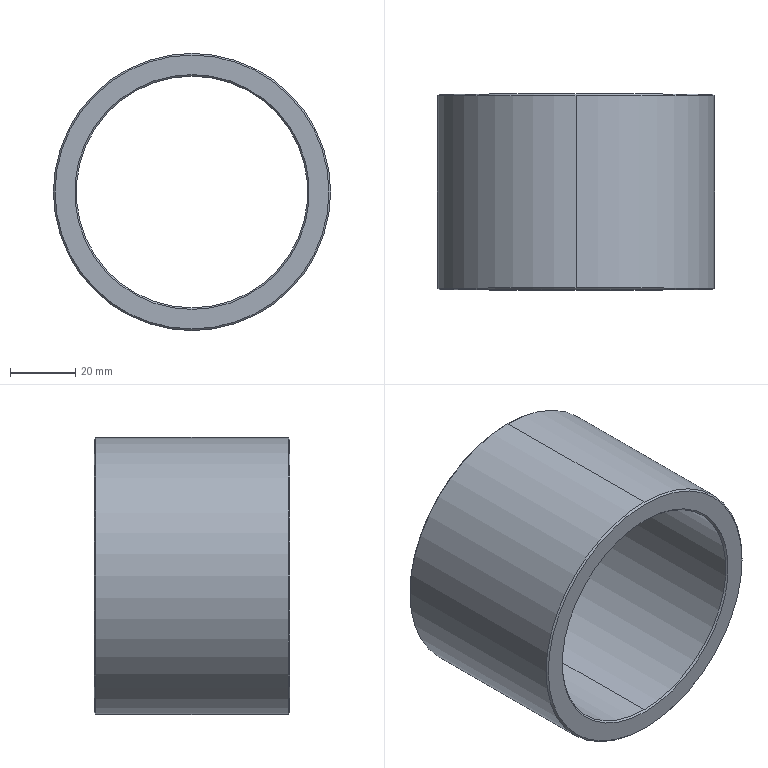Part | SolidWorks | features Chamfer 1, Extrusion 1 | 1 solid | 14 faces | box 85 x 60 x 85 mm | volume 102796 mm3 | cone 8 | cylinder 4 | plane 2 | commonest cylinder face diameters 71 x2 85 x2
STEP:
#1=CARTESIAN_POINT('',(0.,0.5,35.5));
#2=VERTEX_POINT('',#1);
#3=CARTESIAN_POINT('',(0.,0.5,-35.5));
#4=VERTEX_POINT('',#3);
#5=CARTESIAN_POINT('',(0.,0.5,0.));
#6=DIRECTION('',(0.,-1.,0.));
#7=DIRECTION('',(0.,0.,1.));
#8=AXIS2_PLACEMENT_3D('',#5,#6,#7);
#9=CIRCLE('',#8,35.5);
#10=EDGE_CURVE('',#2,#4,#9,.T.);
#11=ORIENTED_EDGE('',*,*,#10,.F.);
#12=CARTESIAN_POINT('',(0.,0.,36.));
#13=VERTEX_POINT('',#12);
#14=CARTESIAN_POINT('',(0.,0.,36.));
#15=DIRECTION('',(0.,-0.7071,0.7071));
#16=VECTOR('',#15,1000.);
#17=LINE('',#14,#16);
#18=EDGE_CURVE('',#2,#13,#17,.T.);
#19=ORIENTED_EDGE('',*,*,#18,.T.);
#20=CARTESIAN_POINT('',(0.,0.,-36.));
#21=VERTEX_POINT('',#20);
#22=CARTESIAN_POINT('',(0.,0.,0.));
#23=DIRECTION('',(0.,1.,0.));
#24=DIRECTION('',(0.,0.,1.));
#25=AXIS2_PLACEMENT_3D('',#22,#23,#24);
#26=CIRCLE('',#25,36.);
#27=EDGE_CURVE('',#21,#13,#26,.T.);
#28=ORIENTED_EDGE('',*,*,#27,.F.);
#29=CARTESIAN_POINT('',(0.,0.,-36.));
#30=DIRECTION('',(0.,-0.7071,-0.7071));
#31=VECTOR('',#30,1000.);
#32=LINE('',#29,#31);
#33=EDGE_CURVE('',#4,#21,#32,.T.);
#34=ORIENTED_EDGE('',*,*,#33,.F.);
#35=EDGE_LOOP('',(#11,#19,#28,#34));
#36=FACE_OUTER_BOUND('',#35,.T.);
#37=CARTESIAN_POINT('',(0.,0.,0.));
#38=DIRECTION('',(0.,-1.,0.));
#39=DIRECTION('',(0.,0.,-1.));
#40=AXIS2_PLACEMENT_3D('',#37,#38,#39);
#41=CONICAL_SURFACE('',#40,36.,0.7854);
#42=ADVANCED_FACE('',(#36),#41,.F.);
#43=CARTESIAN_POINT('',(0.,59.5,-35.5));
#44=VERTEX_POINT('',#43);
#45=CARTESIAN_POINT('',(0.,59.5,35.5));
#46=VERTEX_POINT('',#45);
#47=CARTESIAN_POINT('',(0.,59.5,0.));
#48=DIRECTION('',(0.,1.,0.));
#49=DIRECTION('',(0.,0.,1.));
#50=AXIS2_PLACEMENT_3D('',#47,#48,#49);
#51=CIRCLE('',#50,35.5);
#52=EDGE_CURVE('',#44,#46,#51,.T.);
#53=ORIENTED_EDGE('',*,*,#52,.F.);
#54=CARTESIAN_POINT('',(0.,60.,-36.));
#55=VERTEX_POINT('',#54);
#56=CARTESIAN_POINT('',(0.,59.5,-35.5));
#57=DIRECTION('',(0.,0.7071,-0.7071));
#58=VECTOR('',#57,1000.);
#59=LINE('',#56,#58);
#60=EDGE_CURVE('',#44,#55,#59,.T.);
#61=ORIENTED_EDGE('',*,*,#60,.T.);
#62=CARTESIAN_POINT('',(0.,60.,36.));
#63=VERTEX_POINT('',#62);
#64=CARTESIAN_POINT('',(0.,60.,0.));
#65=DIRECTION('',(0.,-1.,0.));
#66=DIRECTION('',(0.,0.,1.));
#67=AXIS2_PLACEMENT_3D('',#64,#65,#66);
#68=CIRCLE('',#67,36.);
#69=EDGE_CURVE('',#63,#55,#68,.T.);
#70=ORIENTED_EDGE('',*,*,#69,.F.);
#71=CARTESIAN_POINT('',(0.,59.5,35.5));
#72=DIRECTION('',(0.,0.7071,0.7071));
#73=VECTOR('',#72,1000.);
#74=LINE('',#71,#73);
#75=EDGE_CURVE('',#46,#63,#74,.T.);
#76=ORIENTED_EDGE('',*,*,#75,.F.);
#77=EDGE_LOOP('',(#53,#61,#70,#76));
#78=FACE_OUTER_BOUND('',#77,.T.);
#79=CARTESIAN_POINT('',(0.,59.5,0.));
#80=DIRECTION('',(0.,1.,0.));
#81=DIRECTION('',(0.,0.,1.));
#82=AXIS2_PLACEMENT_3D('',#79,#80,#81);
#83=CONICAL_SURFACE('',#82,35.5,0.7854);
#84=ADVANCED_FACE('',(#78),#83,.F.);
#85=CARTESIAN_POINT('',(0.,0.,-42.));
#86=VERTEX_POINT('',#85);
#87=CARTESIAN_POINT('',(0.,0.,42.));
#88=VERTEX_POINT('',#87);
#89=CARTESIAN_POINT('',(0.,0.,0.));
#90=DIRECTION('',(0.,-1.,0.));
#91=DIRECTION('',(0.,0.,1.));
#92=AXIS2_PLACEMENT_3D('',#89,#90,#91);
#93=CIRCLE('',#92,42.);
#94=EDGE_CURVE('',#86,#88,#93,.T.);
#95=ORIENTED_EDGE('',*,*,#94,.F.);
#96=CARTESIAN_POINT('',(0.,0.5,-42.5));
#97=VERTEX_POINT('',#96);
#98=CARTESIAN_POINT('',(0.,0.5,-42.5));
#99=DIRECTION('',(0.,0.7071,-0.7071));
#100=VECTOR('',#99,1000.);
#101=LINE('',#98,#100);
#102=EDGE_CURVE('',#86,#97,#101,.T.);
#103=ORIENTED_EDGE('',*,*,#102,.T.);
#104=CARTESIAN_POINT('',(0.,0.5,42.5));
#105=VERTEX_POINT('',#104);
#106=CARTESIAN_POINT('',(0.,0.5,0.));
#107=DIRECTION('',(0.,1.,0.));
#108=DIRECTION('',(0.,0.,1.));
#109=AXIS2_PLACEMENT_3D('',#106,#107,#108);
#110=CIRCLE('',#109,42.5);
#111=EDGE_CURVE('',#105,#97,#110,.T.);
#112=ORIENTED_EDGE('',*,*,#111,.F.);
#113=CARTESIAN_POINT('',(0.,0.5,42.5));
#114=DIRECTION('',(0.,0.7071,0.7071));
#115=VECTOR('',#114,1000.);
#116=LINE('',#113,#115);
#117=EDGE_CURVE('',#88,#105,#116,.T.);
#118=ORIENTED_EDGE('',*,*,#117,.F.);
#119=EDGE_LOOP('',(#95,#103,#112,#118));
#120=FACE_OUTER_BOUND('',#119,.T.);
#121=CARTESIAN_POINT('',(0.,0.5,0.));
#122=DIRECTION('',(0.,1.,0.));
#123=DIRECTION('',(0.,0.,1.));
#124=AXIS2_PLACEMENT_3D('',#121,#122,#123);
#125=CONICAL_SURFACE('',#124,42.5,0.7854);
#126=ADVANCED_FACE('',(#120),#125,.T.);
#127=CARTESIAN_POINT('',(0.,60.,42.));
#128=VERTEX_POINT('',#127);
#129=CARTESIAN_POINT('',(0.,60.,-42.));
#130=VERTEX_POINT('',#129);
#131=CARTESIAN_POINT('',(0.,60.,0.));
#132=DIRECTION('',(0.,1.,0.));
#133=DIRECTION('',(0.,0.,1.));
#134=AXIS2_PLACEMENT_3D('',#131,#132,#133);
#135=CIRCLE('',#134,42.);
#136=EDGE_CURVE('',#128,#130,#135,.T.);
#137=ORIENTED_EDGE('',*,*,#136,.F.);
#138=CARTESIAN_POINT('',(0.,59.5,42.5));
#139=VERTEX_POINT('',#138);
#140=CARTESIAN_POINT('',(0.,60.,42.));
#141=DIRECTION('',(0.,-0.7071,0.7071));
#142=VECTOR('',#141,1000.);
#143=LINE('',#140,#142);
#144=EDGE_CURVE('',#128,#139,#143,.T.);
#145=ORIENTED_EDGE('',*,*,#144,.T.);
#146=CARTESIAN_POINT('',(0.,59.5,-42.5));
#147=VERTEX_POINT('',#146);
#148=CARTESIAN_POINT('',(0.,59.5,0.));
#149=DIRECTION('',(0.,-1.,0.));
#150=DIRECTION('',(0.,0.,1.));
#151=AXIS2_PLACEMENT_3D('',#148,#149,#150);
#152=CIRCLE('',#151,42.5);
#153=EDGE_CURVE('',#147,#139,#152,.T.);
#154=ORIENTED_EDGE('',*,*,#153,.F.);
#155=CARTESIAN_POINT('',(0.,60.,-42.));
#156=DIRECTION('',(0.,-0.7071,-0.7071));
#157=VECTOR('',#156,1000.);
#158=LINE('',#155,#157);
#159=EDGE_CURVE('',#130,#147,#158,.T.);
#160=ORIENTED_EDGE('',*,*,#159,.F.);
#161=EDGE_LOOP('',(#137,#145,#154,#160));
#162=FACE_OUTER_BOUND('',#161,.T.);
#163=CARTESIAN_POINT('',(0.,60.,0.));
#164=DIRECTION('',(0.,-1.,0.));
#165=DIRECTION('',(0.,0.,-1.));
#166=AXIS2_PLACEMENT_3D('',#163,#164,#165);
#167=CONICAL_SURFACE('',#166,42.,0.7854);
#168=ADVANCED_FACE('',(#162),#167,.T.);
#169=ORIENTED_EDGE('',*,*,#52,.T.);
#170=CARTESIAN_POINT('',(0.,60.,35.5));
#171=DIRECTION('',(0.,-1.,0.));
#172=VECTOR('',#171,1000.);
#173=LINE('',#170,#172);
#174=EDGE_CURVE('',#46,#2,#173,.T.);
#175=ORIENTED_EDGE('',*,*,#174,.T.);
#176=ORIENTED_EDGE('',*,*,#10,.T.);
#177=CARTESIAN_POINT('',(0.,60.,-35.5));
#178=DIRECTION('',(0.,-1.,0.));
#179=VECTOR('',#178,1000.);
#180=LINE('',#177,#179);
#181=EDGE_CURVE('',#44,#4,#180,.T.);
#182=ORIENTED_EDGE('',*,*,#181,.F.);
#183=EDGE_LOOP('',(#169,#175,#176,#182));
#184=FACE_OUTER_BOUND('',#183,.T.);
#185=CARTESIAN_POINT('',(0.,60.,0.));
#186=DIRECTION('',(0.,-1.,0.));
#187=DIRECTION('',(0.,0.,-1.));
#188=AXIS2_PLACEMENT_3D('',#185,#186,#187);
#189=CYLINDRICAL_SURFACE('',#188,35.5);
#190=ADVANCED_FACE('',(#184),#189,.F.);
#191=ORIENTED_EDGE('',*,*,#153,.T.);
#192=CARTESIAN_POINT('',(0.,60.,42.5));
#193=DIRECTION('',(0.,-1.,0.));
#194=VECTOR('',#193,1000.);
#195=LINE('',#192,#194);
#196=EDGE_CURVE('',#139,#105,#195,.T.);
#197=ORIENTED_EDGE('',*,*,#196,.T.);
#198=ORIENTED_EDGE('',*,*,#111,.T.);
#199=CARTESIAN_POINT('',(0.,60.,-42.5));
#200=DIRECTION('',(0.,-1.,0.));
#201=VECTOR('',#200,1000.);
#202=LINE('',#199,#201);
#203=EDGE_CURVE('',#147,#97,#202,.T.);
#204=ORIENTED_EDGE('',*,*,#203,.F.);
#205=EDGE_LOOP('',(#191,#197,#198,#204));
#206=FACE_OUTER_BOUND('',#205,.T.);
#207=CARTESIAN_POINT('',(0.,60.,0.));
#208=DIRECTION('',(0.,-1.,0.));
#209=DIRECTION('',(0.,0.,-1.));
#210=AXIS2_PLACEMENT_3D('',#207,#208,#209);
#211=CYLINDRICAL_SURFACE('',#210,42.5);
#212=ADVANCED_FACE('',(#206),#211,.T.);
#213=CARTESIAN_POINT('',(0.,60.,0.));
#214=DIRECTION('',(0.,1.,0.));
#215=DIRECTION('',(0.,0.,1.));
#216=AXIS2_PLACEMENT_3D('',#213,#214,#215);
#217=CIRCLE('',#216,42.);
#218=EDGE_CURVE('',#130,#128,#217,.T.);
#219=ORIENTED_EDGE('',*,*,#218,.T.);
#220=ORIENTED_EDGE('',*,*,#136,.T.);
#221=EDGE_LOOP('',(#219,#220));
#222=FACE_OUTER_BOUND('',#221,.T.);
#223=ORIENTED_EDGE('',*,*,#69,.T.);
#224=CARTESIAN_POINT('',(0.,60.,0.));
#225=DIRECTION('',(0.,-1.,0.));
#226=DIRECTION('',(0.,0.,1.));
#227=AXIS2_PLACEMENT_3D('',#224,#225,#226);
#228=CIRCLE('',#227,36.);
#229=EDGE_CURVE('',#55,#63,#228,.T.);
#230=ORIENTED_EDGE('',*,*,#229,.T.);
#231=EDGE_LOOP('',(#223,#230));
#232=FACE_BOUND('',#231,.T.);
#233=CARTESIAN_POINT('',(0.,60.,0.));
#234=DIRECTION('',(0.,1.,0.));
#235=DIRECTION('',(0.,0.,1.));
#236=AXIS2_PLACEMENT_3D('',#233,#234,#235);
#237=PLANE('',#236);
#238=ADVANCED_FACE('',(#222,#232),#237,.T.);
#239=CARTESIAN_POINT('',(0.,0.,0.));
#240=DIRECTION('',(0.,-1.,0.));
#241=DIRECTION('',(0.,0.,1.));
#242=AXIS2_PLACEMENT_3D('',#239,#240,#241);
#243=CIRCLE('',#242,42.);
#244=EDGE_CURVE('',#88,#86,#243,.T.);
#245=ORIENTED_EDGE('',*,*,#244,.T.);
#246=ORIENTED_EDGE('',*,*,#94,.T.);
#247=EDGE_LOOP('',(#245,#246));
#248=FACE_OUTER_BOUND('',#247,.T.);
#249=ORIENTED_EDGE('',*,*,#27,.T.);
#250=CARTESIAN_POINT('',(0.,0.,0.));
#251=DIRECTION('',(0.,1.,0.));
#252=DIRECTION('',(0.,0.,1.));
#253=AXIS2_PLACEMENT_3D('',#250,#251,#252);
#254=CIRCLE('',#253,36.);
#255=EDGE_CURVE('',#13,#21,#254,.T.);
#256=ORIENTED_EDGE('',*,*,#255,.T.);
#257=EDGE_LOOP('',(#249,#256));
#258=FACE_BOUND('',#257,.T.);
#259=CARTESIAN_POINT('',(0.,0.,0.));
#260=DIRECTION('',(0.,1.,0.));
#261=DIRECTION('',(0.,0.,1.));
#262=AXIS2_PLACEMENT_3D('',#259,#260,#261);
#263=PLANE('',#262);
#264=ADVANCED_FACE('',(#248,#258),#263,.F.);
#265=ORIENTED_EDGE('',*,*,#196,.F.);
#266=CARTESIAN_POINT('',(0.,59.5,0.));
#267=DIRECTION('',(0.,-1.,0.));
#268=DIRECTION('',(0.,0.,1.));
#269=AXIS2_PLACEMENT_3D('',#266,#267,#268);
#270=CIRCLE('',#269,42.5);
#271=EDGE_CURVE('',#139,#147,#270,.T.);
#272=ORIENTED_EDGE('',*,*,#271,.T.);
#273=ORIENTED_EDGE('',*,*,#203,.T.);
#274=CARTESIAN_POINT('',(0.,0.5,0.));
#275=DIRECTION('',(0.,1.,0.));
#276=DIRECTION('',(0.,0.,1.));
#277=AXIS2_PLACEMENT_3D('',#274,#275,#276);
#278=CIRCLE('',#277,42.5);
#279=EDGE_CURVE('',#97,#105,#278,.T.);
#280=ORIENTED_EDGE('',*,*,#279,.T.);
#281=EDGE_LOOP('',(#265,#272,#273,#280));
#282=FACE_OUTER_BOUND('',#281,.T.);
#283=CARTESIAN_POINT('',(0.,60.,0.));
#284=DIRECTION('',(0.,-1.,0.));
#285=DIRECTION('',(0.,0.,-1.));
#286=AXIS2_PLACEMENT_3D('',#283,#284,#285);
#287=CYLINDRICAL_SURFACE('',#286,42.5);
#288=ADVANCED_FACE('',(#282),#287,.T.);
#289=ORIENTED_EDGE('',*,*,#174,.F.);
#290=CARTESIAN_POINT('',(0.,59.5,0.));
#291=DIRECTION('',(0.,1.,0.));
#292=DIRECTION('',(0.,0.,1.));
#293=AXIS2_PLACEMENT_3D('',#290,#291,#292);
#294=CIRCLE('',#293,35.5);
#295=EDGE_CURVE('',#46,#44,#294,.T.);
#296=ORIENTED_EDGE('',*,*,#295,.T.);
#297=ORIENTED_EDGE('',*,*,#181,.T.);
#298=CARTESIAN_POINT('',(0.,0.5,0.));
#299=DIRECTION('',(0.,-1.,0.));
#300=DIRECTION('',(0.,0.,1.));
#301=AXIS2_PLACEMENT_3D('',#298,#299,#300);
#302=CIRCLE('',#301,35.5);
#303=EDGE_CURVE('',#4,#2,#302,.T.);
#304=ORIENTED_EDGE('',*,*,#303,.T.);
#305=EDGE_LOOP('',(#289,#296,#297,#304));
#306=FACE_OUTER_BOUND('',#305,.T.);
#307=CARTESIAN_POINT('',(0.,60.,0.));
#308=DIRECTION('',(0.,-1.,0.));
#309=DIRECTION('',(0.,0.,-1.));
#310=AXIS2_PLACEMENT_3D('',#307,#308,#309);
#311=CYLINDRICAL_SURFACE('',#310,35.5);
#312=ADVANCED_FACE('',(#306),#311,.F.);
#313=ORIENTED_EDGE('',*,*,#144,.F.);
#314=ORIENTED_EDGE('',*,*,#218,.F.);
#315=ORIENTED_EDGE('',*,*,#159,.T.);
#316=ORIENTED_EDGE('',*,*,#271,.F.);
#317=EDGE_LOOP('',(#313,#314,#315,#316));
#318=FACE_OUTER_BOUND('',#317,.T.);
#319=CARTESIAN_POINT('',(0.,60.,0.));
#320=DIRECTION('',(0.,-1.,0.));
#321=DIRECTION('',(0.,0.,-1.));
#322=AXIS2_PLACEMENT_3D('',#319,#320,#321);
#323=CONICAL_SURFACE('',#322,42.,0.7854);
#324=ADVANCED_FACE('',(#318),#323,.T.);
#325=ORIENTED_EDGE('',*,*,#102,.F.);
#326=ORIENTED_EDGE('',*,*,#244,.F.);
#327=ORIENTED_EDGE('',*,*,#117,.T.);
#328=ORIENTED_EDGE('',*,*,#279,.F.);
#329=EDGE_LOOP('',(#325,#326,#327,#328));
#330=FACE_OUTER_BOUND('',#329,.T.);
#331=CARTESIAN_POINT('',(0.,0.5,0.));
#332=DIRECTION('',(0.,1.,0.));
#333=DIRECTION('',(0.,0.,1.));
#334=AXIS2_PLACEMENT_3D('',#331,#332,#333);
#335=CONICAL_SURFACE('',#334,42.5,0.7854);
#336=ADVANCED_FACE('',(#330),#335,.T.);
#337=ORIENTED_EDGE('',*,*,#60,.F.);
#338=ORIENTED_EDGE('',*,*,#295,.F.);
#339=ORIENTED_EDGE('',*,*,#75,.T.);
#340=ORIENTED_EDGE('',*,*,#229,.F.);
#341=EDGE_LOOP('',(#337,#338,#339,#340));
#342=FACE_OUTER_BOUND('',#341,.T.);
#343=CARTESIAN_POINT('',(0.,59.5,0.));
#344=DIRECTION('',(0.,1.,0.));
#345=DIRECTION('',(0.,0.,1.));
#346=AXIS2_PLACEMENT_3D('',#343,#344,#345);
#347=CONICAL_SURFACE('',#346,35.5,0.7854);
#348=ADVANCED_FACE('',(#342),#347,.F.);
#349=ORIENTED_EDGE('',*,*,#18,.F.);
#350=ORIENTED_EDGE('',*,*,#303,.F.);
#351=ORIENTED_EDGE('',*,*,#33,.T.);
#352=ORIENTED_EDGE('',*,*,#255,.F.);
#353=EDGE_LOOP('',(#349,#350,#351,#352));
#354=FACE_OUTER_BOUND('',#353,.T.);
#355=CARTESIAN_POINT('',(0.,0.,0.));
#356=DIRECTION('',(0.,-1.,0.));
#357=DIRECTION('',(0.,0.,-1.));
#358=AXIS2_PLACEMENT_3D('',#355,#356,#357);
#359=CONICAL_SURFACE('',#358,36.,0.7854);
#360=ADVANCED_FACE('',(#354),#359,.F.);
#361=CLOSED_SHELL('',(#42,#84,#126,#168,#190,#212,#238,#264,#288,#312,#324,#336,#348,#360));
#362=MANIFOLD_SOLID_BREP('',#361);
#363=CARTESIAN_POINT('',(0.,0.,0.));
#364=DIRECTION('',(0.,0.,1.));
#365=DIRECTION('',(1.,0.,0.));
#366=AXIS2_PLACEMENT_3D('',#363,#364,#365);
#367=(LENGTH_UNIT()NAMED_UNIT(*)SI_UNIT(.MILLI.,.METRE.));
#368=UNCERTAINTY_MEASURE_WITH_UNIT(LENGTH_MEASURE(0.00001),#367,'','');
#369=(NAMED_UNIT(*)PLANE_ANGLE_UNIT()SI_UNIT($,.RADIAN.));
#370=(NAMED_UNIT(*)SI_UNIT($,.STERADIAN.)SOLID_ANGLE_UNIT());
#371=(GEOMETRIC_REPRESENTATION_CONTEXT(3)GLOBAL_UNCERTAINTY_ASSIGNED_CONTEXT((#368))GLOBAL_UNIT_ASSIGNED_CONTEXT((#367,#369,#370))REPRESENTATION_CONTEXT('',''));
#372=ADVANCED_BREP_SHAPE_REPRESENTATION('',(#362,#366),#371);